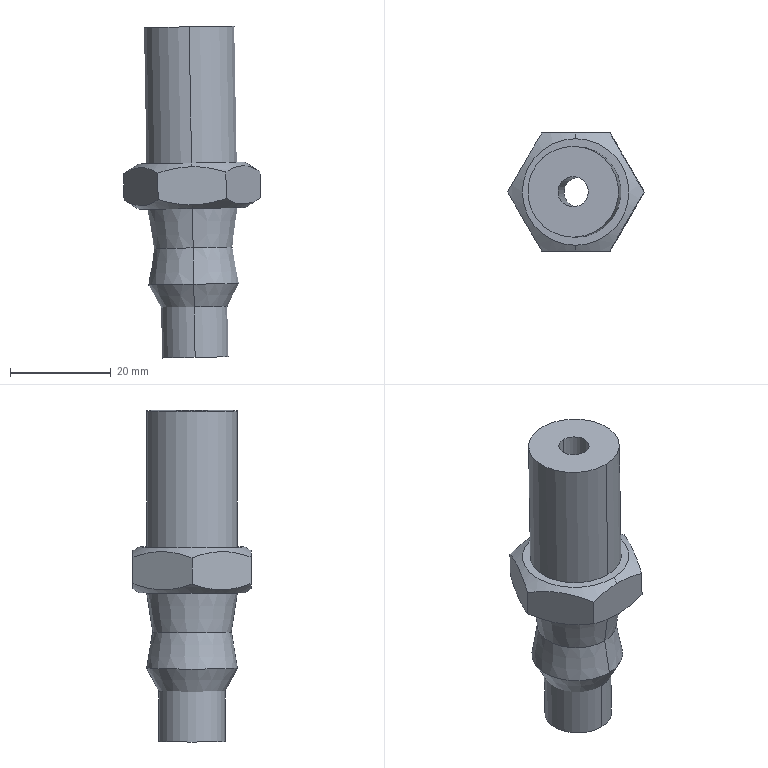Part | STEP file | 2026.6.15-Main Assembly图.sldasm-Part-35 | 1 solid | 27 faces | box 27.111 x 23.4 x 65.773 mm | volume 14698 mm3 | plane 11 | cone 10 | cylinder 6 | commonest cylinder face diameters 6 x2 13.2 x2 18 x2